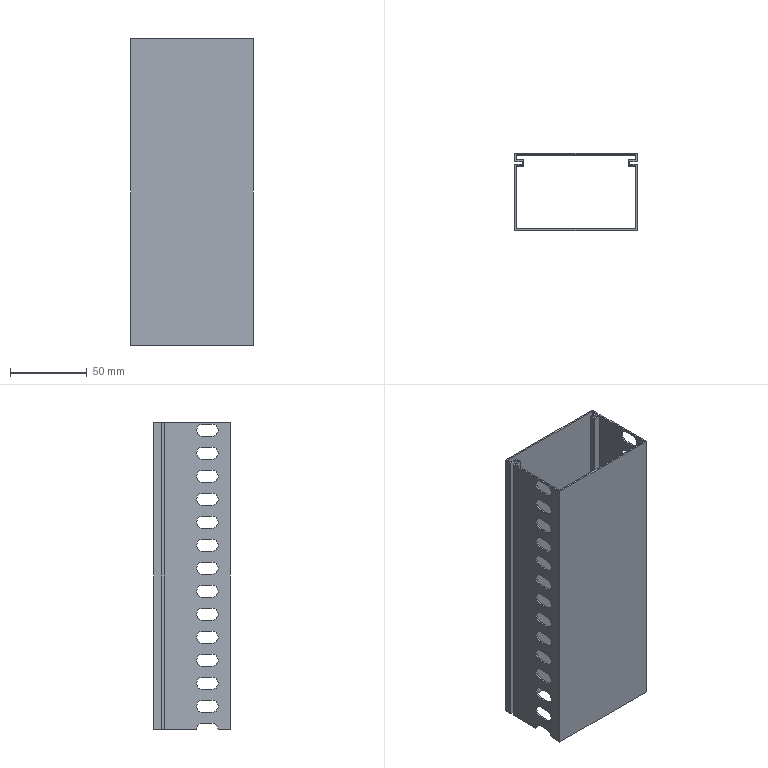Part | SolidWorks | features BaseBody 1 | 1 solid | 137 faces | box 80 x 50 x 200 mm | volume 52547 mm3 | plane 81 | cylinder 56 | commonest cylinder face diameters 8 x56